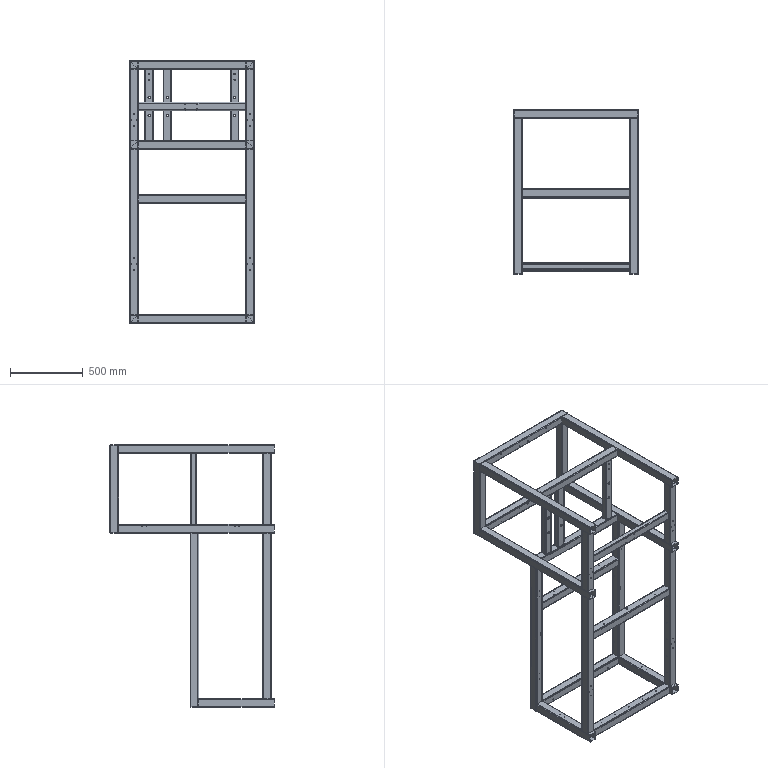Part | STEP file | JBJ-P-1006-01_Default<As Machined> | 26 solids | 618 faces | box 860 x 1133 x 1810 mm | volume 13158479 mm3 | cylinder 358 | plane 260 | commonest cylinder face diameters 6 x104 12 x104 5 x92 2.5 x28 8.5 x16 17 x12